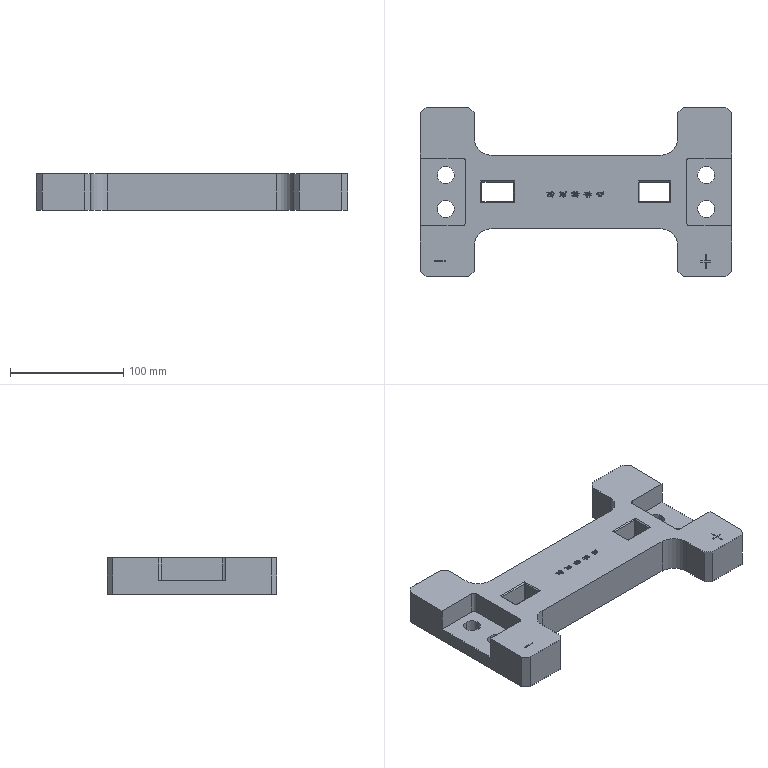NC program | NX | posted with a generic post | part box 275 x 150 x 32 mm
Lines 1 to 1365 of 10049:
N10 G17 G21 G94 G90
(FLOOR_WALL , TOOL : D17R0.8)
N12 T21 M6
N14 G54
N16 G17 G0 G90 X-147.5 Y-6.755 S2000 M3
N18 G43 Z30. H21
N20 Z1.172
N22 G94 G1 Z-0.328 F1000.
N24 X-138.35 Y-1.472
N26 G3 X-137.5 Y0. R1.7
N28 G1 Y21.35 F2000.
N30 X-106.15
N32 Y-21.35
N34 X-137.5
N36 Y0.
N38 X-129.
N40 Y12.85
N42 X-114.65
N44 Y-12.85
N46 X-129.
N48 Y0.
N50 G3 X-129.85 Y1.472 R1.7
N52 G1 Z1.172
N54 G0 X-147.5 Y-6.755 Z0.843
N56 G1 Z-0.657 F1000.
N58 X-138.35 Y-1.472
N60 G3 X-137.5 Y0. R1.7
N62 G1 Y21.35 F2000.
N64 X-106.15
N66 Y-21.35
N68 X-137.5
N70 Y0.
N72 X-129.
N74 Y12.85
N76 X-114.65
N78 Y-12.85
N80 X-129.
N82 Y0.
N84 G3 X-129.85 Y1.472 R1.7
N86 G1 Z0.843
N88 G0 X-147.5 Y-6.755 Z0.515
N90 G1 Z-0.985 F1000.
N92 X-138.35 Y-1.472
N94 G3 X-137.5 Y0. R1.7
N96 G1 Y21.35 F2000.
N98 X-106.15
N100 Y-21.35
N102 X-137.5
N104 Y0.
N106 X-129.
N108 Y12.85
N110 X-114.65
N112 Y-12.85
N114 X-129.
N116 Y0.
N118 G3 X-129.85 Y1.472 R1.7
N120 G1 Z0.515
N122 G0 X-147.5 Y-6.755 Z0.187
N124 G1 Z-1.313 F1000.
N126 X-138.35 Y-1.472
N128 G3 X-137.5 Y0. R1.7
N130 G1 Y21.35 F2000.
N132 X-106.15
N134 Y-21.35
N136 X-137.5
N138 Y0.
N140 X-129.
N142 Y12.85
N144 X-114.65
N146 Y-12.85
N148 X-129.
N150 Y0.
N152 G3 X-129.85 Y1.472 R1.7
N154 G1 Z0.187
N156 G0 X-147.5 Y-6.755 Z-0.142
N158 G1 Z-1.642 F1000.
N160 X-138.35 Y-1.472
N162 G3 X-137.5 Y0. R1.7
N164 G1 Y21.35 F2000.
N166 X-106.15
N168 Y-21.35
N170 X-137.5
N172 Y0.
N174 X-129.
N176 Y12.85
N178 X-114.65
N180 Y-12.85
N182 X-129.
N184 Y0.
N186 G3 X-129.85 Y1.472 R1.7
N188 G1 Z-0.142
N190 G0 X-147.5 Y-6.755 Z-0.47
N192 G1 Z-1.97 F1000.
N194 X-138.35 Y-1.472
N196 G3 X-137.5 Y0. R1.7
N198 G1 Y21.35 F2000.
N200 X-106.15
N202 Y-21.35
N204 X-137.5
N206 Y0.
N208 X-129.
N210 Y12.85
N212 X-114.65
N214 Y-12.85
N216 X-129.
N218 Y0.
N220 G3 X-129.85 Y1.472 R1.7
N222 G1 Z-0.47
N224 G0 X-147.5 Y-6.755 Z-0.798
N226 G1 Z-2.298 F1000.
N228 X-138.35 Y-1.472
N230 G3 X-137.5 Y0. R1.7
N232 G1 Y21.35 F2000.
N234 X-106.15
N236 Y-21.35
N238 X-137.5
N240 Y0.
N242 X-129.
N244 Y12.85
N246 X-114.65
N248 Y-12.85
N250 X-129.
N252 Y0.
N254 G3 X-129.85 Y1.472 R1.7
N256 G1 Z-0.798
N258 G0 X-147.5 Y-6.755 Z-1.127
N260 G1 Z-2.627 F1000.
N262 X-138.35 Y-1.472
N264 G3 X-137.5 Y0. R1.7
N266 G1 Y21.35 F2000.
N268 X-106.15
N270 Y-21.35
N272 X-137.5
N274 Y0.
N276 X-129.
N278 Y12.85
N280 X-114.65
N282 Y-12.85
N284 X-129.
N286 Y0.
N288 G3 X-129.85 Y1.472 R1.7
N290 G1 Z-1.127
N292 G0 X-147.5 Y-6.755 Z-1.455
N294 G1 Z-2.955 F1000.
N296 X-138.35 Y-1.472
N298 G3 X-137.5 Y0. R1.7
N300 G1 Y21.35 F2000.
N302 X-106.15
N304 Y-21.35
N306 X-137.5
N308 Y0.
N310 X-129.
N312 Y12.85
N314 X-114.65
N316 Y-12.85
N318 X-129.
N320 Y0.
N322 G3 X-129.85 Y1.472 R1.7
N324 G1 Z-1.455
N326 G0 X-147.5 Y-6.755 Z-1.783
N328 G1 Z-3.283 F1000.
N330 X-138.35 Y-1.472
N332 G3 X-137.5 Y0. R1.7
N334 G1 Y21.35 F2000.
N336 X-106.15
N338 Y-21.35
N340 X-137.5
N342 Y0.
N344 X-129.
N346 Y12.85
N348 X-114.65
N350 Y-12.85
N352 X-129.
N354 Y0.
N356 G3 X-129.85 Y1.472 R1.7
N358 G1 Z-1.783
N360 G0 X-147.5 Y-6.755 Z-2.112
N362 G1 Z-3.612 F1000.
N364 X-138.35 Y-1.472
N366 G3 X-137.5 Y0. R1.7
N368 G1 Y21.35 F2000.
N370 X-106.15
N372 Y-21.35
N374 X-137.5
N376 Y0.
N378 X-129.
N380 Y12.85
N382 X-114.65
N384 Y-12.85
N386 X-129.
N388 Y0.
N390 G3 X-129.85 Y1.472 R1.7
N392 G1 Z-2.112
N394 G0 X-147.5 Y-6.755 Z-2.44
N396 G1 Z-3.94 F1000.
N398 X-138.35 Y-1.472
N400 G3 X-137.5 Y0. R1.7
N402 G1 Y21.35 F2000.
N404 X-106.15
N406 Y-21.35
N408 X-137.5
N410 Y0.
N412 X-129.
N414 Y12.85
N416 X-114.65
N418 Y-12.85
N420 X-129.
N422 Y0.
N424 G3 X-129.85 Y1.472 R1.7
N426 G1 Z-2.44
N428 G0 X-147.5 Y-6.755 Z-2.768
N430 G1 Z-4.268 F1000.
N432 X-138.35 Y-1.472
N434 G3 X-137.5 Y0. R1.7
N436 G1 Y21.35 F2000.
N438 X-106.15
N440 Y-21.35
N442 X-137.5
N444 Y0.
N446 X-129.
N448 Y12.85
N450 X-114.65
N452 Y-12.85
N454 X-129.
N456 Y0.
N458 G3 X-129.85 Y1.472 R1.7
N460 G1 Z-2.768
N462 G0 X-147.5 Y-6.755 Z-3.097
N464 G1 Z-4.597 F1000.
N466 X-138.35 Y-1.472
N468 G3 X-137.5 Y0. R1.7
N470 G1 Y21.35 F2000.
N472 X-106.15
N474 Y-21.35
N476 X-137.5
N478 Y0.
N480 X-129.
N482 Y12.85
N484 X-114.65
N486 Y-12.85
N488 X-129.
N490 Y0.
N492 G3 X-129.85 Y1.472 R1.7
N494 G1 Z-3.097
N496 G0 X-147.5 Y-6.755 Z-3.425
N498 G1 Z-4.925 F1000.
N500 X-138.35 Y-1.472
N502 G3 X-137.5 Y0. R1.7
N504 G1 Y21.35 F2000.
N506 X-106.15
N508 Y-21.35
N510 X-137.5
N512 Y0.
N514 X-129.
N516 Y12.85
N518 X-114.65
N520 Y-12.85
N522 X-129.
N524 Y0.
N526 G3 X-129.85 Y1.472 R1.7
N528 G1 Z-3.425
N530 G0 X-147.5 Y-6.755 Z-3.753
N532 G1 Z-5.253 F1000.
N534 X-138.35 Y-1.472
N536 G3 X-137.5 Y0. R1.7
N538 G1 Y21.35 F2000.
N540 X-106.15
N542 Y-21.35
N544 X-137.5
N546 Y0.
N548 X-129.
N550 Y12.85
N552 X-114.65
N554 Y-12.85
N556 X-129.
N558 Y0.
N560 G3 X-129.85 Y1.472 R1.7
N562 G1 Z-3.753
N564 G0 X-147.5 Y-6.755 Z-4.082
N566 G1 Z-5.582 F1000.
N568 X-138.35 Y-1.472
N570 G3 X-137.5 Y0. R1.7
N572 G1 Y21.35 F2000.
N574 X-106.15
N576 Y-21.35
N578 X-137.5
N580 Y0.
N582 X-129.
N584 Y12.85
N586 X-114.65
N588 Y-12.85
N590 X-129.
N592 Y0.
N594 G3 X-129.85 Y1.472 R1.7
N596 G1 Z-4.082
N598 G0 X-147.5 Y-6.755 Z-4.41
N600 G1 Z-5.91 F1000.
N602 X-138.35 Y-1.472
N604 G3 X-137.5 Y0. R1.7
N606 G1 Y21.35 F2000.
N608 X-106.15
N610 Y-21.35
N612 X-137.5
N614 Y0.
N616 X-129.
N618 Y12.85
N620 X-114.65
N622 Y-12.85
N624 X-129.
N626 Y0.
N628 G3 X-129.85 Y1.472 R1.7
N630 G1 Z-4.41
N632 G0 X-147.5 Y-6.755 Z-4.738
N634 G1 Z-6.238 F1000.
N636 X-138.35 Y-1.472
N638 G3 X-137.5 Y0. R1.7
N640 G1 Y21.35 F2000.
N642 X-106.15
N644 Y-21.35
N646 X-137.5
N648 Y0.
N650 X-129.
N652 Y12.85
N654 X-114.65
N656 Y-12.85
N658 X-129.
N660 Y0.
N662 G3 X-129.85 Y1.472 R1.7
N664 G1 Z-4.738
N666 G0 X-147.5 Y-6.755 Z-5.067
N668 G1 Z-6.567 F1000.
N670 X-138.35 Y-1.472
N672 G3 X-137.5 Y0. R1.7
N674 G1 Y21.35 F2000.
N676 X-106.15
N678 Y-21.35
N680 X-137.5
N682 Y0.
N684 X-129.
N686 Y12.85
N688 X-114.65
N690 Y-12.85
N692 X-129.
N694 Y0.
N696 G3 X-129.85 Y1.472 R1.7
N698 G1 Z-5.067
N700 G0 X-147.5 Y-6.755 Z-5.395
N702 G1 Z-6.895 F1000.
N704 X-138.35 Y-1.472
N706 G3 X-137.5 Y0. R1.7
N708 G1 Y21.35 F2000.
N710 X-106.15
N712 Y-21.35
N714 X-137.5
N716 Y0.
N718 X-129.
N720 Y12.85
N722 X-114.65
N724 Y-12.85
N726 X-129.
N728 Y0.
N730 G3 X-129.85 Y1.472 R1.7
N732 G1 Z-5.395
N734 G0 X-147.5 Y-6.755 Z-5.723
N736 G1 Z-7.223 F1000.
N738 X-138.35 Y-1.472
N740 G3 X-137.5 Y0. R1.7
N742 G1 Y21.35 F2000.
N744 X-106.15
N746 Y-21.35
N748 X-137.5
N750 Y0.
N752 X-129.
N754 Y12.85
N756 X-114.65
N758 Y-12.85
N760 X-129.
N762 Y0.
N764 G3 X-129.85 Y1.472 R1.7
N766 G1 Z-5.723
N768 G0 X-147.5 Y-6.755 Z-6.052
N770 G1 Z-7.552 F1000.
N772 X-138.35 Y-1.472
N774 G3 X-137.5 Y0. R1.7
N776 G1 Y21.35 F2000.
N778 X-106.15
N780 Y-21.35
N782 X-137.5
N784 Y0.
N786 X-129.
N788 Y12.85
N790 X-114.65
N792 Y-12.85
N794 X-129.
N796 Y0.
N798 G3 X-129.85 Y1.472 R1.7
N800 G1 Z-6.052
N802 G0 X-147.5 Y-6.755 Z-6.38
N804 G1 Z-7.88 F1000.
N806 X-138.35 Y-1.472
N808 G3 X-137.5 Y0. R1.7
N810 G1 Y21.35 F2000.
N812 X-106.15
N814 Y-21.35
N816 X-137.5
N818 Y0.
N820 X-129.
N822 Y12.85
N824 X-114.65
N826 Y-12.85
N828 X-129.
N830 Y0.
N832 G3 X-129.85 Y1.472 R1.7
N834 G1 Z-6.38
N836 G0 X-147.5 Y-6.755 Z-6.708
N838 G1 Z-8.208 F1000.
N840 X-138.35 Y-1.472
N842 G3 X-137.5 Y0. R1.7
N844 G1 Y21.35 F2000.
N846 X-106.15
N848 Y-21.35
N850 X-137.5
N852 Y0.
N854 X-129.
N856 Y12.85
N858 X-114.65
N860 Y-12.85
N862 X-129.
N864 Y0.
N866 G3 X-129.85 Y1.472 R1.7
N868 G1 Z-6.708
N870 G0 X-147.5 Y-6.755 Z-7.037
N872 G1 Z-8.537 F1000.
N874 X-138.35 Y-1.472
N876 G3 X-137.5 Y0. R1.7
N878 G1 Y21.35 F2000.
N880 X-106.15
N882 Y-21.35
N884 X-137.5
N886 Y0.
N888 X-129.
N890 Y12.85
N892 X-114.65
N894 Y-12.85
N896 X-129.
N898 Y0.
N900 G3 X-129.85 Y1.472 R1.7
N902 G1 Z-7.037
N904 G0 X-147.5 Y-6.755 Z-7.365
N906 G1 Z-8.865 F1000.
N908 X-138.35 Y-1.472
N910 G3 X-137.5 Y0. R1.7
N912 G1 Y21.35 F2000.
N914 X-106.15
N916 Y-21.35
N918 X-137.5
N920 Y0.
N922 X-129.
N924 Y12.85
N926 X-114.65
N928 Y-12.85
N930 X-129.
N932 Y0.
N934 G3 X-129.85 Y1.472 R1.7
N936 G1 Z-7.365
N938 G0 X-147.5 Y-6.755 Z-7.693
N940 G1 Z-9.193 F1000.
N942 X-138.35 Y-1.472
N944 G3 X-137.5 Y0. R1.7
N946 G1 Y21.35 F2000.
N948 X-106.15
N950 Y-21.35
N952 X-137.5
N954 Y0.
N956 X-129.
N958 Y12.85
N960 X-114.65
N962 Y-12.85
N964 X-129.
N966 Y0.
N968 G3 X-129.85 Y1.472 R1.7
N970 G1 Z-7.693
N972 G0 X-147.5 Y-6.755 Z-8.022
N974 G1 Z-9.522 F1000.
N976 X-138.35 Y-1.472
N978 G3 X-137.5 Y0. R1.7
N980 G1 Y21.35 F2000.
N982 X-106.15
N984 Y-21.35
N986 X-137.5
N988 Y0.
N990 X-129.
N992 Y12.85
N994 X-114.65
N996 Y-12.85
N998 X-129.
N1000 Y0.
N1002 G3 X-129.85 Y1.472 R1.7
N1004 G1 Z-8.022
N1006 G0 X-147.5 Y-6.755 Z-8.35
N1008 G1 Z-9.85 F1000.
N1010 X-138.35 Y-1.472
N1012 G3 X-137.5 Y0. R1.7
N1014 G1 Y21.35 F2000.
N1016 X-106.15
N1018 Y-21.35
N1020 X-137.5
N1022 Y0.
N1024 X-129.
N1026 Y12.85
N1028 X-114.65
N1030 Y-12.85
N1032 X-129.
N1034 Y0.
N1036 G3 X-129.85 Y1.472 R1.7
N1038 G1 Z-8.35
N1040 G0 X-147.5 Y-6.755 Z-8.678
N1042 G1 Z-10.178 F1000.
N1044 X-138.35 Y-1.472
N1046 G3 X-137.5 Y0. R1.7
N1048 G1 Y21.35 F2000.
N1050 X-106.15
N1052 Y-21.35
N1054 X-137.5
N1056 Y0.
N1058 X-129.
N1060 Y12.85
N1062 X-114.65
N1064 Y-12.85
N1066 X-129.
N1068 Y0.
N1070 G3 X-129.85 Y1.472 R1.7
N1072 G1 Z-8.678
N1074 G0 X-147.5 Y-6.755 Z-9.007
N1076 G1 Z-10.507 F1000.
N1078 X-138.35 Y-1.472
N1080 G3 X-137.5 Y0. R1.7
N1082 G1 Y21.35 F2000.
N1084 X-106.15
N1086 Y-21.35
N1088 X-137.5
N1090 Y0.
N1092 X-129.
N1094 Y12.85
N1096 X-114.65
N1098 Y-12.85
N1100 X-129.
N1102 Y0.
N1104 G3 X-129.85 Y1.472 R1.7
N1106 G1 Z-9.007
N1108 G0 X-147.5 Y-6.755 Z-9.335
N1110 G1 Z-10.835 F1000.
N1112 X-138.35 Y-1.472
N1114 G3 X-137.5 Y0. R1.7
N1116 G1 Y21.35 F2000.
N1118 X-106.15
N1120 Y-21.35
N1122 X-137.5
N1124 Y0.
N1126 X-129.
N1128 Y12.85
N1130 X-114.65
N1132 Y-12.85
N1134 X-129.
N1136 Y0.
N1138 G3 X-129.85 Y1.472 R1.7
N1140 G1 Z-9.335
N1142 G0 X-147.5 Y-6.755 Z-9.663
N1144 G1 Z-11.163 F1000.
N1146 X-138.35 Y-1.472
N1148 G3 X-137.5 Y0. R1.7
N1150 G1 Y21.35 F2000.
N1152 X-106.15
N1154 Y-21.35
N1156 X-137.5
N1158 Y0.
N1160 X-129.
N1162 Y12.85
N1164 X-114.65
N1166 Y-12.85
N1168 X-129.
N1170 Y0.
N1172 G3 X-129.85 Y1.472 R1.7
N1174 G1 Z-9.663
N1176 G0 X-147.5 Y-6.755 Z-9.992
N1178 G1 Z-11.492 F1000.
N1180 X-138.35 Y-1.472
N1182 G3 X-137.5 Y0. R1.7
N1184 G1 Y21.35 F2000.
N1186 X-106.15
N1188 Y-21.35
N1190 X-137.5
N1192 Y0.
N1194 X-129.
N1196 Y12.85
N1198 X-114.65
N1200 Y-12.85
N1202 X-129.
N1204 Y0.
N1206 G3 X-129.85 Y1.472 R1.7
N1208 G1 Z-9.992
N1210 G0 X-147.5 Y-6.755 Z-10.32
N1212 G1 Z-11.82 F1000.
N1214 X-138.35 Y-1.472
N1216 G3 X-137.5 Y0. R1.7
N1218 G1 Y21.35 F2000.
N1220 X-106.15
N1222 Y-21.35
N1224 X-137.5
N1226 Y0.
N1228 X-129.
N1230 Y12.85
N1232 X-114.65
N1234 Y-12.85
N1236 X-129.
N1238 Y0.
N1240 G3 X-129.85 Y1.472 R1.7
N1242 G1 Z-10.32
N1244 G0 X-147.5 Y-6.755 Z-10.648
N1246 G1 Z-12.148 F1000.
N1248 X-138.35 Y-1.472
N1250 G3 X-137.5 Y0. R1.7
N1252 G1 Y21.35 F2000.
N1254 X-106.15
N1256 Y-21.35
N1258 X-137.5
N1260 Y0.
N1262 X-129.
N1264 Y12.85
N1266 X-114.65
N1268 Y-12.85
N1270 X-129.
N1272 Y0.
N1274 G3 X-129.85 Y1.472 R1.7
N1276 G1 Z-10.648
N1278 G0 X-147.5 Y-6.755 Z-10.977
N1280 G1 Z-12.477 F1000.
N1282 X-138.35 Y-1.472
N1284 G3 X-137.5 Y0. R1.7
N1286 G1 Y21.35 F2000.
N1288 X-106.15
N1290 Y-21.35
N1292 X-137.5
N1294 Y0.
N1296 X-129.
N1298 Y12.85
N1300 X-114.65
N1302 Y-12.85
N1304 X-129.
N1306 Y0.
N1308 G3 X-129.85 Y1.472 R1.7
N1310 G1 Z-10.977
N1312 G0 X-147.5 Y-6.755 Z-11.305
N1314 G1 Z-12.805 F1000.
N1316 X-138.35 Y-1.472
N1318 G3 X-137.5 Y0. R1.7
N1320 G1 Y21.35 F2000.
N1322 X-106.15
N1324 Y-21.35
N1326 X-137.5
N1328 Y0.
N1330 X-129.
N1332 Y12.85
N1334 X-114.65
N1336 Y-12.85
N1338 X-129.
N1340 Y0.
N1342 G3 X-129.85 Y1.472 R1.7
N1344 G1 Z-11.305
N1346 G0 X-147.5 Y-6.755 Z-11.633
N1348 G1 Z-13.133 F1000.
N1350 X-138.35 Y-1.472
N1352 G3 X-137.5 Y0. R1.7
N1354 G1 Y21.35 F2000.
N1356 X-106.15
N1358 Y-21.35
N1360 X-137.5
N1362 Y0.
N1364 X-129.
N1366 Y12.85
N1368 X-114.65
N1370 Y-12.85
N1372 X-129.
N1374 Y0.
N1376 G3 X-129.85 Y1.472 R1.7
N1378 G1 Z-11.633
N1380 G0 X-147.5 Y-6.755 Z-11.962
N1382 G1 Z-13.462 F1000.
N1384 X-138.35 Y-1.472
N1386 G3 X-137.5 Y0. R1.7
N1388 G1 Y21.35 F2000.
N1390 X-106.15
N1392 Y-21.35
N1394 X-137.5
N1396 Y0.
N1398 X-129.
N1400 Y12.85
N1402 X-114.65
N1404 Y-12.85
N1406 X-129.
N1408 Y0.
N1410 G3 X-129.85 Y1.472 R1.7
N1412 G1 Z-11.962
N1414 G0 X-147.5 Y-6.755 Z-12.29
N1416 G1 Z-13.79 F1000.
N1418 X-138.35 Y-1.472
N1420 G3 X-137.5 Y0. R1.7
N1422 G1 Y21.35 F2000.
N1424 X-106.15
N1426 Y-21.35
N1428 X-137.5
N1430 Y0.
N1432 X-129.
N1434 Y12.85
N1436 X-114.65
N1438 Y-12.85
N1440 X-129.
N1442 Y0.
N1444 G3 X-129.85 Y1.472 R1.7
N1446 G1 Z-12.29
N1448 G0 X-147.5 Y-6.755 Z-12.618
N1450 G1 Z-14.118 F1000.
N1452 X-138.35 Y-1.472
N1454 G3 X-137.5 Y0. R1.7
N1456 G1 Y21.35 F2000.
N1458 X-106.15
N1460 Y-21.35
N1462 X-137.5
N1464 Y0.
N1466 X-129.
N1468 Y12.85
N1470 X-114.65
N1472 Y-12.85
N1474 X-129.
N1476 Y0.
N1478 G3 X-129.85 Y1.472 R1.7
N1480 G1 Z-12.618
N1482 G0 X-147.5 Y-6.755 Z-12.947
N1484 G1 Z-14.447 F1000.
N1486 X-138.35 Y-1.472
N1488 G3 X-137.5 Y0. R1.7
N1490 G1 Y21.35 F2000.
N1492 X-106.15
N1494 Y-21.35
N1496 X-137.5
N1498 Y0.
N1500 X-129.
N1502 Y12.85
N1504 X-114.65
N1506 Y-12.85
N1508 X-129.
N1510 Y0.
N1512 G3 X-129.85 Y1.472 R1.7
N1514 G1 Z-12.947
N1516 G0 X-147.5 Y-6.755 Z-13.275
N1518 G1 Z-14.775 F1000.
N1520 X-138.35 Y-1.472
N1522 G3 X-137.5 Y0. R1.7
N1524 G1 Y21.35 F2000.
N1526 X-106.15
N1528 Y-21.35
N1530 X-137.5
N1532 Y0.
N1534 X-129.
N1536 Y12.85
N1538 X-114.65
N1540 Y-12.85
N1542 X-129.
N1544 Y0.
N1546 G3 X-129.85 Y1.472 R1.7
N1548 G1 Z-13.275
N1550 G0 X-147.5 Y-6.755 Z-13.603
N1552 G1 Z-15.103 F1000.
N1554 X-138.35 Y-1.472
N1556 G3 X-137.5 Y0. R1.7
N1558 G1 Y21.35 F2000.
N1560 X-106.15
N1562 Y-21.35
N1564 X-137.5
N1566 Y0.
N1568 X-129.
N1570 Y12.85
N1572 X-114.65
N1574 Y-12.85
N1576 X-129.
N1578 Y0.
N1580 G3 X-129.85 Y1.472 R1.7
N1582 G1 Z-13.603
N1584 G0 X-147.5 Y-6.755 Z-13.932
N1586 G1 Z-15.432 F1000.
N1588 X-138.35 Y-1.472
N1590 G3 X-137.5 Y0. R1.7
N1592 G1 Y21.35 F2000.
N1594 X-106.15
N1596 Y-21.35
N1598 X-137.5
N1600 Y0.
N1602 X-129.
N1604 Y12.85
N1606 X-114.65
N1608 Y-12.85
N1610 X-129.
N1612 Y0.
N1614 G3 X-129.85 Y1.472 R1.7
N1616 G1 Z-13.932
N1618 G0 X-147.5 Y-6.755 Z-14.26
N1620 G1 Z-15.76 F1000.
N1622 X-138.35 Y-1.472
N1624 G3 X-137.5 Y0. R1.7
N1626 G1 Y21.35 F2000.
N1628 X-106.15
N1630 Y-21.35
N1632 X-137.5
N1634 Y0.
N1636 X-129.
N1638 Y12.85
N1640 X-114.65
N1642 Y-12.85
N1644 X-129.
N1646 Y0.
N1648 G3 X-129.85 Y1.472 R1.7
N1650 G1 Z-14.26
N1652 G0 X-147.5 Y-6.755 Z-14.588
N1654 G1 Z-16.088 F1000.
N1656 X-138.35 Y-1.472
N1658 G3 X-137.5 Y0. R1.7
N1660 G1 Y21.35 F2000.
N1662 X-106.15
N1664 Y-21.35
N1666 X-137.5
N1668 Y0.
N1670 X-129.
N1672 Y12.85
N1674 X-114.65
N1676 Y-12.85
N1678 X-129.
N1680 Y0.
N1682 G3 X-129.85 Y1.472 R1.7
N1684 G1 Z-14.588
N1686 G0 X-147.5 Y-6.755 Z-14.917
N1688 G1 Z-16.417 F1000.
N1690 X-138.35 Y-1.472
N1692 G3 X-137.5 Y0. R1.7
N1694 G1 Y21.35 F2000.
N1696 X-106.15
N1698 Y-21.35
N1700 X-137.5
N1702 Y0.
N1704 X-129.
N1706 Y12.85
N1708 X-114.65
N1710 Y-12.85
N1712 X-129.
N1714 Y0.
N1716 G3 X-129.85 Y1.472 R1.7
N1718 G1 Z-14.917
N1720 G0 X-147.5 Y-6.755 Z-15.245
N1722 G1 Z-16.745 F1000.
N1724 X-138.35 Y-1.472
N1726 G3 X-137.5 Y0. R1.7
N1728 G1 Y21.35 F2000.
N1730 X-106.15
N1732 Y-21.35
N1734 X-137.5
N1736 Y0.
N1738 X-129.
N1740 Y12.85
N1742 X-114.65
N1744 Y-12.85
N1746 X-129.
N1748 Y0.
N1750 G3 X-129.85 Y1.472 R1.7
N1752 G1 Z-15.245
N1754 G0 X-147.5 Y-6.755 Z-15.573
N1756 G1 Z-17.073 F1000.
N1758 X-138.35 Y-1.472
N1760 G3 X-137.5 Y0. R1.7
N1762 G1 Y21.35 F2000.
N1764 X-106.15
N1766 Y-21.35
N1768 X-137.5
N1770 Y0.
N1772 X-129.
N1774 Y12.85
N1776 X-114.65
N1778 Y-12.85
N1780 X-129.
N1782 Y0.
N1784 G3 X-129.85 Y1.472 R1.7
N1786 G1 Z-15.573
N1788 G0 X-147.5 Y-6.755 Z-15.902
N1790 G1 Z-17.402 F1000.
N1792 X-138.35 Y-1.472
N1794 G3 X-137.5 Y0. R1.7
N1796 G1 Y21.35 F2000.
N1798 X-106.15
N1800 Y-21.35
N1802 X-137.5
N1804 Y0.
N1806 X-129.
N1808 Y12.85
N1810 X-114.65
N1812 Y-12.85
N1814 X-129.
N1816 Y0.
N1818 G3 X-129.85 Y1.472 R1.7
N1820 G1 Z-15.902
N1822 G0 X-147.5 Y-6.755 Z-16.23
N1824 G1 Z-17.73 F1000.
N1826 X-138.35 Y-1.472
N1828 G3 X-137.5 Y0. R1.7
N1830 G1 Y21.35 F2000.
N1832 X-106.15
N1834 Y-21.35
N1836 X-137.5
N1838 Y0.
N1840 X-129.
N1842 Y12.85
N1844 X-114.65
N1846 Y-12.85
N1848 X-129.
N1850 Y0.
N1852 G3 X-129.85 Y1.472 R1.7
N1854 G1 Z-16.23
N1856 G0 X-147.5 Y-6.755 Z-16.558
N1858 G1 Z-18.058 F1000.
N1860 X-138.35 Y-1.472
N1862 G3 X-137.5 Y0. R1.7
N1864 G1 Y21.35 F2000.
N1866 X-106.15
N1868 Y-21.35
N1870 X-137.5
N1872 Y0.
N1874 X-129.
N1876 Y12.85
N1878 X-114.65
N1880 Y-12.85
N1882 X-129.
N1884 Y0.
N1886 G3 X-129.85 Y1.472 R1.7
N1888 G1 Z-16.558
N1890 G0 X-147.5 Y-6.755 Z-16.887
N1892 G1 Z-18.387 F1000.
N1894 X-138.35 Y-1.472
N1896 G3 X-137.5 Y0. R1.7
N1898 G1 Y21.35 F2000.
N1900 X-106.15
N1902 Y-21.35
N1904 X-137.5
N1906 Y0.
N1908 X-129.
N1910 Y12.85
N1912 X-114.65
N1914 Y-12.85
N1916 X-129.
N1918 Y0.
N1920 G3 X-129.85 Y1.472 R1.7
N1922 G1 Z-16.887
N1924 G0 X-147.5 Y-6.755 Z-17.215
N1926 G1 Z-18.715 F1000.
N1928 X-138.35 Y-1.472
N1930 G3 X-137.5 Y0. R1.7
N1932 G1 Y21.35 F2000.
N1934 X-106.15
N1936 Y-21.35
N1938 X-137.5
N1940 Y0.
N1942 X-129.
N1944 Y12.85
N1946 X-114.65
N1948 Y-12.85
N1950 X-129.
N1952 Y0.
N1954 G3 X-129.85 Y1.472 R1.7
N1956 G1 Z-17.215
N1958 G0 X-147.5 Y-6.755 Z-17.543
N1960 G1 Z-19.043 F1000.
N1962 X-138.35 Y-1.472
N1964 G3 X-137.5 Y0. R1.7
N1966 G1 Y21.35 F2000.
N1968 X-106.15
N1970 Y-21.35
N1972 X-137.5
N1974 Y0.
N1976 X-129.
N1978 Y12.85
N1980 X-114.65
N1982 Y-12.85
N1984 X-129.
N1986 Y0.
N1988 G3 X-129.85 Y1.472 R1.7
N1990 G1 Z-17.543
N1992 G0 X-147.5 Y-6.755 Z-17.872
N1994 G1 Z-19.372 F1000.
N1996 X-138.35 Y-1.472
N1998 G3 X-137.5 Y0. R1.7
N2000 G1 Y21.35 F2000.
N2002 X-106.15
N2004 Y-21.35
N2006 X-137.5
N2008 Y0.
N2010 X-129.
N2012 Y12.85
N2014 X-114.65
N2016 Y-12.85
N2018 X-129.
N2020 Y0.
N2022 G3 X-129.85 Y1.472 R1.7
N2024 G1 Z-17.872
N2026 G0 X-147.5 Y-6.755 Z-18.2
N2028 G1 Z-19.7 F1000.
N2030 X-138.35 Y-1.472
N2032 G3 X-137.5 Y0. R1.7
N2034 G1 Y21.35 F2000.
N2036 X-106.15
N2038 Y-21.35
N2040 X-137.5
N2042 Y0.
N2044 X-129.
N2046 Y12.85
N2048 X-114.65
N2050 Y-12.85
N2052 X-129.
N2054 Y0.
N2056 G3 X-129.85 Y1.472 R1.7
N2058 G1 Z-18.2
N2060 G0 Z30.
N2062 X147.5 Y6.755
N2064 Z1.172
N2066 G1 Z-0.328 F1000.
N2068 X138.35 Y1.472
N2070 G3 X137.5 Y0. R1.7
N2072 G1 Y-21.35 F2000.
N2074 X106.15
N2076 Y21.35
N2078 X137.5
N2080 Y0.
N2082 X129.
N2084 Y-12.85
N2086 X114.65
N2088 Y12.85
N2090 X129.
N2092 Y0.
N2094 G3 X129.85 Y-1.472 R1.7
N2096 G1 Z1.172
N2098 G0 X147.5 Y6.755 Z0.843
N2100 G1 Z-0.657 F1000.
N2102 X138.35 Y1.472
N2104 G3 X137.5 Y0. R1.7
N2106 G1 Y-21.35 F2000.
N2108 X106.15
N2110 Y21.35
N2112 X137.5
N2114 Y0.
N2116 X129.
N2118 Y-12.85
N2120 X114.65
N2122 Y12.85
N2124 X129.
N2126 Y0.
N2128 G3 X129.85 Y-1.472 R1.7
N2130 G1 Z0.843
N2132 G0 X147.5 Y6.755 Z0.515
N2134 G1 Z-0.985 F1000.
N2136 X138.35 Y1.472
N2138 G3 X137.5 Y0. R1.7
N2140 G1 Y-21.35 F2000.
N2142 X106.15
N2144 Y21.35
N2146 X137.5
N2148 Y0.
N2150 X129.
N2152 Y-12.85
N2154 X114.65
N2156 Y12.85
N2158 X129.
N2160 Y0.
N2162 G3 X129.85 Y-1.472 R1.7
N2164 G1 Z0.515
N2166 G0 X147.5 Y6.755 Z0.187
N2168 G1 Z-1.313 F1000.
N2170 X138.35 Y1.472
N2172 G3 X137.5 Y0. R1.7
N2174 G1 Y-21.35 F2000.
N2176 X106.15
N2178 Y21.35
N2180 X137.5
N2182 Y0.
N2184 X129.
N2186 Y-12.85
N2188 X114.65
N2190 Y12.85
N2192 X129.
N2194 Y0.
N2196 G3 X129.85 Y-1.472 R1.7
N2198 G1 Z0.187
N2200 G0 X147.5 Y6.755 Z-0.142
N2202 G1 Z-1.642 F1000.
N2204 X138.35 Y1.472
N2206 G3 X137.5 Y0. R1.7
N2208 G1 Y-21.35 F2000.
N2210 X106.15
N2212 Y21.35
N2214 X137.5
N2216 Y0.
N2218 X129.
N2220 Y-12.85
N2222 X114.65
N2224 Y12.85
N2226 X129.
N2228 Y0.
N2230 G3 X129.85 Y-1.472 R1.7
N2232 G1 Z-0.142
N2234 G0 X147.5 Y6.755 Z-0.47
N2236 G1 Z-1.97 F1000.
N2238 X138.35 Y1.472
N2240 G3 X137.5 Y0. R1.7
N2242 G1 Y-21.35 F2000.
N2244 X106.15
N2246 Y21.35
N2248 X137.5
N2250 Y0.
N2252 X129.
N2254 Y-12.85
N2256 X114.65
N2258 Y12.85
N2260 X129.
N2262 Y0.
N2264 G3 X129.85 Y-1.472 R1.7
N2266 G1 Z-0.47
N2268 G0 X147.5 Y6.755 Z-0.798
N2270 G1 Z-2.298 F1000.
N2272 X138.35 Y1.472
N2274 G3 X137.5 Y0. R1.7
N2276 G1 Y-21.35 F2000.
N2278 X106.15
N2280 Y21.35
N2282 X137.5
N2284 Y0.
N2286 X129.
N2288 Y-12.85
N2290 X114.65
N2292 Y12.85
N2294 X129.
N2296 Y0.
N2298 G3 X129.85 Y-1.472 R1.7
N2300 G1 Z-0.798
N2302 G0 X147.5 Y6.755 Z-1.127
N2304 G1 Z-2.627 F1000.
N2306 X138.35 Y1.472
N2308 G3 X137.5 Y0. R1.7
N2310 G1 Y-21.35 F2000.
N2312 X106.15
N2314 Y21.35
N2316 X137.5
N2318 Y0.
N2320 X129.
N2322 Y-12.85
N2324 X114.65
N2326 Y12.85
N2328 X129.
N2330 Y0.
N2332 G3 X129.85 Y-1.472 R1.7
N2334 G1 Z-1.127
N2336 G0 X147.5 Y6.755 Z-1.455
N2338 G1 Z-2.955 F1000.
N2340 X138.35 Y1.472
N2342 G3 X137.5 Y0. R1.7
N2344 G1 Y-21.35 F2000.
N2346 X106.15
N2348 Y21.35
N2350 X137.5
N2352 Y0.
N2354 X129.
N2356 Y-12.85
N2358 X114.65
N2360 Y12.85
N2362 X129.
N2364 Y0.
N2366 G3 X129.85 Y-1.472 R1.7
N2368 G1 Z-1.455
N2370 G0 X147.5 Y6.755 Z-1.783
N2372 G1 Z-3.283 F1000.
N2374 X138.35 Y1.472
N2376 G3 X137.5 Y0. R1.7
N2378 G1 Y-21.35 F2000.
N2380 X106.15
N2382 Y21.35
N2384 X137.5
N2386 Y0.
N2388 X129.
N2390 Y-12.85
N2392 X114.65
N2394 Y12.85
N2396 X129.
N2398 Y0.
N2400 G3 X129.85 Y-1.472 R1.7
N2402 G1 Z-1.783
N2404 G0 X147.5 Y6.755 Z-2.112
N2406 G1 Z-3.612 F1000.
N2408 X138.35 Y1.472
N2410 G3 X137.5 Y0. R1.7
N2412 G1 Y-21.35 F2000.
N2414 X106.15
N2416 Y21.35
N2418 X137.5
N2420 Y0.
N2422 X129.
N2424 Y-12.85
N2426 X114.65
N2428 Y12.85
N2430 X129.
N2432 Y0.
N2434 G3 X129.85 Y-1.472 R1.7
N2436 G1 Z-2.112
N2438 G0 X147.5 Y6.755 Z-2.44
N2440 G1 Z-3.94 F1000.
N2442 X138.35 Y1.472
N2444 G3 X137.5 Y0. R1.7
N2446 G1 Y-21.35 F2000.
N2448 X106.15
N2450 Y21.35
N2452 X137.5
N2454 Y0.
N2456 X129.
N2458 Y-12.85
N2460 X114.65
N2462 Y12.85
N2464 X129.
N2466 Y0.
N2468 G3 X129.85 Y-1.472 R1.7
N2470 G1 Z-2.44
N2472 G0 X147.5 Y6.755 Z-2.768
N2474 G1 Z-4.268 F1000.
N2476 X138.35 Y1.472
N2478 G3 X137.5 Y0. R1.7
N2480 G1 Y-21.35 F2000.
N2482 X106.15
N2484 Y21.35
N2486 X137.5
N2488 Y0.
N2490 X129.
N2492 Y-12.85
N2494 X114.65
N2496 Y12.85
N2498 X129.
N2500 Y0.
N2502 G3 X129.85 Y-1.472 R1.7
N2504 G1 Z-2.768
N2506 G0 X147.5 Y6.755 Z-3.097
N2508 G1 Z-4.597 F1000.
N2510 X138.35 Y1.472
N2512 G3 X137.5 Y0. R1.7
N2514 G1 Y-21.35 F2000.
N2516 X106.15
N2518 Y21.35
N2520 X137.5
N2522 Y0.
N2524 X129.
N2526 Y-12.85
N2528 X114.65
N2530 Y12.85
N2532 X129.
N2534 Y0.
N2536 G3 X129.85 Y-1.472 R1.7
N2538 G1 Z-3.097
N2540 G0 X147.5 Y6.755 Z-3.425
N2542 G1 Z-4.925 F1000.
N2544 X138.35 Y1.472
N2546 G3 X137.5 Y0. R1.7
N2548 G1 Y-21.35 F2000.
N2550 X106.15
N2552 Y21.35
N2554 X137.5
N2556 Y0.
N2558 X129.
N2560 Y-12.85
N2562 X114.65
N2564 Y12.85
N2566 X129.
N2568 Y0.
N2570 G3 X129.85 Y-1.472 R1.7
N2572 G1 Z-3.425
N2574 G0 X147.5 Y6.755 Z-3.753
N2576 G1 Z-5.253 F1000.
N2578 X138.35 Y1.472
N2580 G3 X137.5 Y0. R1.7
N2582 G1 Y-21.35 F2000.
N2584 X106.15
N2586 Y21.35
N2588 X137.5
N2590 Y0.
N2592 X129.
N2594 Y-12.85
N2596 X114.65
N2598 Y12.85
N2600 X129.
N2602 Y0.
N2604 G3 X129.85 Y-1.472 R1.7
N2606 G1 Z-3.753
N2608 G0 X147.5 Y6.755 Z-4.082
N2610 G1 Z-5.582 F1000.
N2612 X138.35 Y1.472
N2614 G3 X137.5 Y0. R1.7
N2616 G1 Y-21.35 F2000.
N2618 X106.15
N2620 Y21.35
N2622 X137.5
N2624 Y0.
N2626 X129.
N2628 Y-12.85
N2630 X114.65
N2632 Y12.85
N2634 X129.
N2636 Y0.
N2638 G3 X129.85 Y-1.472 R1.7
N2640 G1 Z-4.082
N2642 G0 X147.5 Y6.755 Z-4.41
N2644 G1 Z-5.91 F1000.
N2646 X138.35 Y1.472
N2648 G3 X137.5 Y0. R1.7
N2650 G1 Y-21.35 F2000.
N2652 X106.15
N2654 Y21.35
N2656 X137.5
N2658 Y0.
N2660 X129.
N2662 Y-12.85
N2664 X114.65
N2666 Y12.85
N2668 X129.
N2670 Y0.
N2672 G3 X129.85 Y-1.472 R1.7
N2674 G1 Z-4.41
N2676 G0 X147.5 Y6.755 Z-4.738
N2678 G1 Z-6.238 F1000.
N2680 X138.35 Y1.472
N2682 G3 X137.5 Y0. R1.7
N2684 G1 Y-21.35 F2000.
N2686 X106.15
N2688 Y21.35
N2690 X137.5
N2692 Y0.
N2694 X129.
N2696 Y-12.85
N2698 X114.65
N2700 Y12.85
N2702 X129.
N2704 Y0.
N2706 G3 X129.85 Y-1.472 R1.7
N2708 G1 Z-4.738
N2710 G0 X147.5 Y6.755 Z-5.067
N2712 G1 Z-6.567 F1000.
N2714 X138.35 Y1.472
N2716 G3 X137.5 Y0. R1.7
N2718 G1 Y-21.35 F2000.
N2720 X106.15
N2722 Y21.35
N2724 X137.5
N2726 Y0.
N2728 X129.